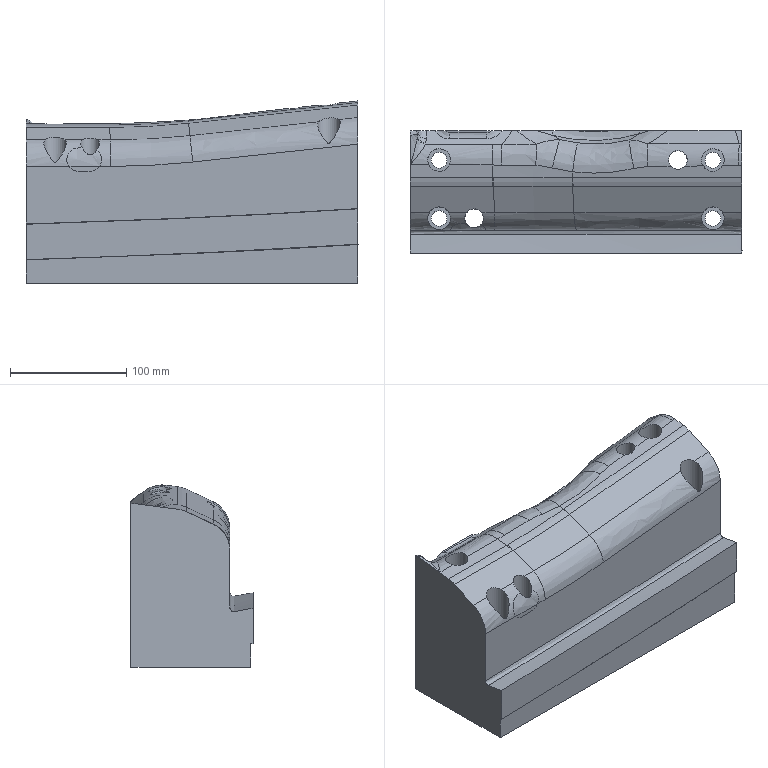Part | NX | features solid 2 | 1 solid | 78 faces | box 285 x 104.828 x 156.414 mm | volume 3353908 mm3 | spline 60 | cylinder 10 | plane 8 | commonest cylinder face diameters 13.5 x4 19.5 x4 16 x2